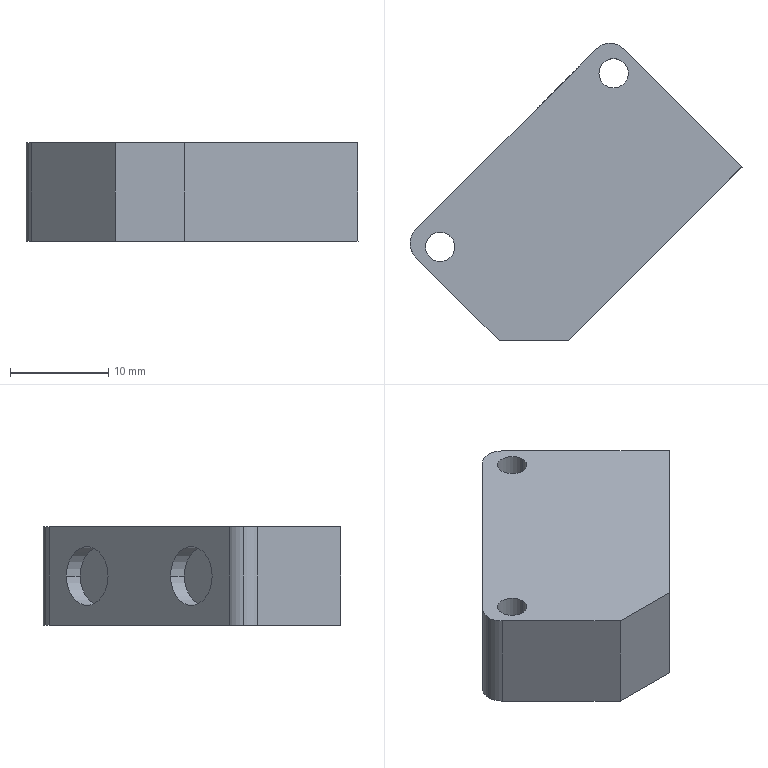Part | SolidWorks | features BaseBody 1 | 1 solid | 20 faces | box 33.82 x 30.284 x 10 mm | volume 5303 mm3 | cylinder 11 | plane 9 | commonest cylinder face diameters 3 x4 6 x4 4 x3
STEP:
#1=CARTESIAN_POINT('',(390.202,1591.211,-336.822));
#2=VERTEX_POINT('',#1);
#3=CARTESIAN_POINT('',(387.202,1591.211,-336.822));
#4=VERTEX_POINT('',#3);
#5=CARTESIAN_POINT('',(388.702,1591.211,-336.822));
#6=DIRECTION('',(0.,0.,-1.));
#7=DIRECTION('',(-1.,0.,0.));
#8=AXIS2_PLACEMENT_3D('',#5,#6,#7);
#9=CIRCLE('',#8,1.5);
#10=EDGE_CURVE('',#2,#4,#9,.T.);
#11=ORIENTED_EDGE('',*,*,#10,.F.);
#12=CARTESIAN_POINT('',(390.202,1591.211,-346.822));
#13=VERTEX_POINT('',#12);
#14=CARTESIAN_POINT('',(390.202,1591.211,-336.822));
#15=DIRECTION('',(0.,0.,-1.));
#16=VECTOR('',#15,1000.);
#17=LINE('',#14,#16);
#18=EDGE_CURVE('',#2,#13,#17,.T.);
#19=ORIENTED_EDGE('',*,*,#18,.T.);
#20=CARTESIAN_POINT('',(387.202,1591.211,-346.822));
#21=VERTEX_POINT('',#20);
#22=CARTESIAN_POINT('',(388.702,1591.211,-346.822));
#23=DIRECTION('',(0.,0.,-1.));
#24=DIRECTION('',(-1.,0.,0.));
#25=AXIS2_PLACEMENT_3D('',#22,#23,#24);
#26=CIRCLE('',#25,1.5);
#27=EDGE_CURVE('',#13,#21,#26,.T.);
#28=ORIENTED_EDGE('',*,*,#27,.T.);
#29=CARTESIAN_POINT('',(387.202,1591.211,-336.822));
#30=DIRECTION('',(0.,0.,-1.));
#31=VECTOR('',#30,1000.);
#32=LINE('',#29,#31);
#33=EDGE_CURVE('',#4,#21,#32,.T.);
#34=ORIENTED_EDGE('',*,*,#33,.F.);
#35=EDGE_LOOP('',(#11,#19,#28,#34));
#36=FACE_OUTER_BOUND('',#35,.T.);
#37=CARTESIAN_POINT('',(388.702,1591.211,-336.822));
#38=DIRECTION('',(0.,0.,-1.));
#39=DIRECTION('',(-1.,0.,0.));
#40=AXIS2_PLACEMENT_3D('',#37,#38,#39);
#41=CYLINDRICAL_SURFACE('',#40,1.5);
#42=ADVANCED_FACE('',(#36),#41,.F.);
#43=CARTESIAN_POINT('',(407.879,1608.889,-336.822));
#44=VERTEX_POINT('',#43);
#45=CARTESIAN_POINT('',(404.879,1608.889,-336.822));
#46=VERTEX_POINT('',#45);
#47=CARTESIAN_POINT('',(406.379,1608.889,-336.822));
#48=DIRECTION('',(0.,0.,-1.));
#49=DIRECTION('',(-1.,0.,0.));
#50=AXIS2_PLACEMENT_3D('',#47,#48,#49);
#51=CIRCLE('',#50,1.5);
#52=EDGE_CURVE('',#44,#46,#51,.T.);
#53=ORIENTED_EDGE('',*,*,#52,.F.);
#54=CARTESIAN_POINT('',(407.879,1608.889,-346.822));
#55=VERTEX_POINT('',#54);
#56=CARTESIAN_POINT('',(407.879,1608.889,-336.822));
#57=DIRECTION('',(0.,0.,-1.));
#58=VECTOR('',#57,1000.);
#59=LINE('',#56,#58);
#60=EDGE_CURVE('',#44,#55,#59,.T.);
#61=ORIENTED_EDGE('',*,*,#60,.T.);
#62=CARTESIAN_POINT('',(404.879,1608.889,-346.822));
#63=VERTEX_POINT('',#62);
#64=CARTESIAN_POINT('',(406.379,1608.889,-346.822));
#65=DIRECTION('',(0.,0.,-1.));
#66=DIRECTION('',(-1.,0.,0.));
#67=AXIS2_PLACEMENT_3D('',#64,#65,#66);
#68=CIRCLE('',#67,1.5);
#69=EDGE_CURVE('',#55,#63,#68,.T.);
#70=ORIENTED_EDGE('',*,*,#69,.T.);
#71=CARTESIAN_POINT('',(404.879,1608.889,-336.822));
#72=DIRECTION('',(0.,0.,-1.));
#73=VECTOR('',#72,1000.);
#74=LINE('',#71,#73);
#75=EDGE_CURVE('',#46,#63,#74,.T.);
#76=ORIENTED_EDGE('',*,*,#75,.F.);
#77=EDGE_LOOP('',(#53,#61,#70,#76));
#78=FACE_OUTER_BOUND('',#77,.T.);
#79=CARTESIAN_POINT('',(406.379,1608.889,-336.822));
#80=DIRECTION('',(0.,0.,-1.));
#81=DIRECTION('',(-1.,0.,0.));
#82=AXIS2_PLACEMENT_3D('',#79,#80,#81);
#83=CYLINDRICAL_SURFACE('',#82,1.5);
#84=ADVANCED_FACE('',(#78),#83,.F.);
#85=CARTESIAN_POINT('',(386.227,1590.151,-336.822));
#86=VERTEX_POINT('',#85);
#87=CARTESIAN_POINT('',(385.641,1591.565,-336.822));
#88=VERTEX_POINT('',#87);
#89=CARTESIAN_POINT('',(387.641,1591.565,-336.822));
#90=DIRECTION('',(0.,0.,-1.));
#91=DIRECTION('',(-1.,0.,0.));
#92=AXIS2_PLACEMENT_3D('',#89,#90,#91);
#93=CIRCLE('',#92,2.);
#94=EDGE_CURVE('',#86,#88,#93,.T.);
#95=ORIENTED_EDGE('',*,*,#94,.T.);
#96=CARTESIAN_POINT('',(385.641,1591.565,-346.822));
#97=VERTEX_POINT('',#96);
#98=CARTESIAN_POINT('',(385.641,1591.565,-336.822));
#99=DIRECTION('',(0.,0.,-1.));
#100=VECTOR('',#99,1000.);
#101=LINE('',#98,#100);
#102=EDGE_CURVE('',#88,#97,#101,.T.);
#103=ORIENTED_EDGE('',*,*,#102,.T.);
#104=CARTESIAN_POINT('',(386.227,1590.151,-346.822));
#105=VERTEX_POINT('',#104);
#106=CARTESIAN_POINT('',(387.641,1591.565,-346.822));
#107=DIRECTION('',(0.,0.,1.));
#108=DIRECTION('',(-1.,0.,0.));
#109=AXIS2_PLACEMENT_3D('',#106,#107,#108);
#110=CIRCLE('',#109,2.);
#111=EDGE_CURVE('',#97,#105,#110,.T.);
#112=ORIENTED_EDGE('',*,*,#111,.T.);
#113=CARTESIAN_POINT('',(386.227,1590.151,-336.822));
#114=DIRECTION('',(0.,0.,1.));
#115=VECTOR('',#114,1000.);
#116=LINE('',#113,#115);
#117=EDGE_CURVE('',#105,#86,#116,.T.);
#118=ORIENTED_EDGE('',*,*,#117,.T.);
#119=EDGE_LOOP('',(#95,#103,#112,#118));
#120=FACE_OUTER_BOUND('',#119,.T.);
#121=CARTESIAN_POINT('',(387.641,1591.565,-336.822));
#122=DIRECTION('',(0.,0.,-1.));
#123=DIRECTION('',(-1.,0.,0.));
#124=AXIS2_PLACEMENT_3D('',#121,#122,#123);
#125=CYLINDRICAL_SURFACE('',#124,2.);
#126=ADVANCED_FACE('',(#120),#125,.T.);
#127=CARTESIAN_POINT('',(404.258,1608.182,-341.822));
#128=VERTEX_POINT('',#127);
#129=CARTESIAN_POINT('',(400.015,1603.939,-341.822));
#130=VERTEX_POINT('',#129);
#131=CARTESIAN_POINT('',(402.137,1606.061,-341.822));
#132=DIRECTION('',(-0.7071,0.7071,0.));
#133=DIRECTION('',(-0.7071,-0.7071,0.));
#134=AXIS2_PLACEMENT_3D('',#131,#132,#133);
#135=CIRCLE('',#134,3.);
#136=EDGE_CURVE('',#128,#130,#135,.T.);
#137=ORIENTED_EDGE('',*,*,#136,.F.);
#138=CARTESIAN_POINT('',(402.844,1609.596,-341.822));
#139=VERTEX_POINT('',#138);
#140=CARTESIAN_POINT('',(404.258,1608.182,-341.822));
#141=DIRECTION('',(-0.7071,0.7071,0.));
#142=VECTOR('',#141,1000.);
#143=LINE('',#140,#142);
#144=EDGE_CURVE('',#128,#139,#143,.T.);
#145=ORIENTED_EDGE('',*,*,#144,.T.);
#146=CARTESIAN_POINT('',(398.601,1605.353,-341.822));
#147=VERTEX_POINT('',#146);
#148=CARTESIAN_POINT('',(400.722,1607.475,-341.822));
#149=DIRECTION('',(-0.7071,0.7071,0.));
#150=DIRECTION('',(-0.7071,-0.7071,0.));
#151=AXIS2_PLACEMENT_3D('',#148,#149,#150);
#152=CIRCLE('',#151,3.);
#153=EDGE_CURVE('',#139,#147,#152,.T.);
#154=ORIENTED_EDGE('',*,*,#153,.T.);
#155=CARTESIAN_POINT('',(400.015,1603.939,-341.822));
#156=DIRECTION('',(-0.7071,0.7071,0.));
#157=VECTOR('',#156,1000.);
#158=LINE('',#155,#157);
#159=EDGE_CURVE('',#130,#147,#158,.T.);
#160=ORIENTED_EDGE('',*,*,#159,.F.);
#161=EDGE_LOOP('',(#137,#145,#154,#160));
#162=FACE_OUTER_BOUND('',#161,.T.);
#163=CARTESIAN_POINT('',(402.137,1606.061,-341.822));
#164=DIRECTION('',(-0.7071,0.7071,0.));
#165=DIRECTION('',(-0.7071,-0.7071,0.));
#166=AXIS2_PLACEMENT_3D('',#163,#164,#165);
#167=CYLINDRICAL_SURFACE('',#166,3.);
#168=ADVANCED_FACE('',(#162),#167,.F.);
#169=CARTESIAN_POINT('',(393.651,1597.575,-341.822));
#170=VERTEX_POINT('',#169);
#171=CARTESIAN_POINT('',(389.409,1593.333,-341.822));
#172=VERTEX_POINT('',#171);
#173=CARTESIAN_POINT('',(391.53,1595.454,-341.822));
#174=DIRECTION('',(-0.7071,0.7071,0.));
#175=DIRECTION('',(-0.7071,-0.7071,0.));
#176=AXIS2_PLACEMENT_3D('',#173,#174,#175);
#177=CIRCLE('',#176,3.);
#178=EDGE_CURVE('',#170,#172,#177,.T.);
#179=ORIENTED_EDGE('',*,*,#178,.F.);
#180=CARTESIAN_POINT('',(392.237,1598.989,-341.822));
#181=VERTEX_POINT('',#180);
#182=CARTESIAN_POINT('',(393.651,1597.575,-341.822));
#183=DIRECTION('',(-0.7071,0.7071,0.));
#184=VECTOR('',#183,1000.);
#185=LINE('',#182,#184);
#186=EDGE_CURVE('',#170,#181,#185,.T.);
#187=ORIENTED_EDGE('',*,*,#186,.T.);
#188=CARTESIAN_POINT('',(387.994,1594.747,-341.822));
#189=VERTEX_POINT('',#188);
#190=CARTESIAN_POINT('',(390.116,1596.868,-341.822));
#191=DIRECTION('',(-0.7071,0.7071,0.));
#192=DIRECTION('',(-0.7071,-0.7071,0.));
#193=AXIS2_PLACEMENT_3D('',#190,#191,#192);
#194=CIRCLE('',#193,3.);
#195=EDGE_CURVE('',#181,#189,#194,.T.);
#196=ORIENTED_EDGE('',*,*,#195,.T.);
#197=CARTESIAN_POINT('',(389.409,1593.333,-341.822));
#198=DIRECTION('',(-0.7071,0.7071,0.));
#199=VECTOR('',#198,1000.);
#200=LINE('',#197,#199);
#201=EDGE_CURVE('',#172,#189,#200,.T.);
#202=ORIENTED_EDGE('',*,*,#201,.F.);
#203=EDGE_LOOP('',(#179,#187,#196,#202));
#204=FACE_OUTER_BOUND('',#203,.T.);
#205=CARTESIAN_POINT('',(391.53,1595.454,-341.822));
#206=DIRECTION('',(-0.7071,0.7071,0.));
#207=DIRECTION('',(-0.7071,-0.7071,0.));
#208=AXIS2_PLACEMENT_3D('',#205,#206,#207);
#209=CYLINDRICAL_SURFACE('',#208,3.);
#210=ADVANCED_FACE('',(#204),#209,.F.);
#211=CARTESIAN_POINT('',(388.702,1591.211,-346.822));
#212=DIRECTION('',(0.,0.,-1.));
#213=DIRECTION('',(-1.,0.,0.));
#214=AXIS2_PLACEMENT_3D('',#211,#212,#213);
#215=CIRCLE('',#214,1.5);
#216=EDGE_CURVE('',#21,#13,#215,.T.);
#217=ORIENTED_EDGE('',*,*,#216,.F.);
#218=ORIENTED_EDGE('',*,*,#27,.F.);
#219=EDGE_LOOP('',(#217,#218));
#220=FACE_BOUND('',#219,.T.);
#221=CARTESIAN_POINT('',(406.379,1608.889,-346.822));
#222=DIRECTION('',(0.,0.,-1.));
#223=DIRECTION('',(-1.,0.,0.));
#224=AXIS2_PLACEMENT_3D('',#221,#222,#223);
#225=CIRCLE('',#224,1.5);
#226=EDGE_CURVE('',#63,#55,#225,.T.);
#227=ORIENTED_EDGE('',*,*,#226,.F.);
#228=ORIENTED_EDGE('',*,*,#69,.F.);
#229=EDGE_LOOP('',(#227,#228));
#230=FACE_BOUND('',#229,.T.);
#231=CARTESIAN_POINT('',(401.783,1581.665,-346.822));
#232=VERTEX_POINT('',#231);
#233=CARTESIAN_POINT('',(419.461,1599.343,-346.822));
#234=VERTEX_POINT('',#233);
#235=CARTESIAN_POINT('',(401.783,1581.665,-346.822));
#236=DIRECTION('',(0.7071,0.7071,0.));
#237=VECTOR('',#236,1000.);
#238=LINE('',#235,#237);
#239=EDGE_CURVE('',#232,#234,#238,.T.);
#240=ORIENTED_EDGE('',*,*,#239,.F.);
#241=CARTESIAN_POINT('',(394.712,1581.665,-346.822));
#242=VERTEX_POINT('',#241);
#243=CARTESIAN_POINT('',(406.026,1581.665,-346.822));
#244=DIRECTION('',(1.,0.,0.));
#245=VECTOR('',#244,1000.);
#246=LINE('',#243,#245);
#247=EDGE_CURVE('',#242,#232,#246,.T.);
#248=ORIENTED_EDGE('',*,*,#247,.F.);
#249=CARTESIAN_POINT('',(386.227,1590.151,-346.822));
#250=DIRECTION('',(0.7071,-0.7071,0.));
#251=VECTOR('',#250,1000.);
#252=LINE('',#249,#251);
#253=EDGE_CURVE('',#105,#242,#252,.T.);
#254=ORIENTED_EDGE('',*,*,#253,.F.);
#255=ORIENTED_EDGE('',*,*,#111,.F.);
#256=CARTESIAN_POINT('',(386.227,1592.979,-346.822));
#257=VERTEX_POINT('',#256);
#258=CARTESIAN_POINT('',(387.641,1591.565,-346.822));
#259=DIRECTION('',(0.,0.,1.));
#260=DIRECTION('',(-1.,0.,0.));
#261=AXIS2_PLACEMENT_3D('',#258,#259,#260);
#262=CIRCLE('',#261,2.);
#263=EDGE_CURVE('',#257,#97,#262,.T.);
#264=ORIENTED_EDGE('',*,*,#263,.F.);
#265=CARTESIAN_POINT('',(404.612,1611.364,-346.822));
#266=VERTEX_POINT('',#265);
#267=CARTESIAN_POINT('',(404.612,1611.364,-346.822));
#268=DIRECTION('',(-0.7071,-0.7071,0.));
#269=VECTOR('',#268,1000.);
#270=LINE('',#267,#269);
#271=EDGE_CURVE('',#266,#257,#270,.T.);
#272=ORIENTED_EDGE('',*,*,#271,.F.);
#273=CARTESIAN_POINT('',(407.44,1611.364,-346.822));
#274=VERTEX_POINT('',#273);
#275=CARTESIAN_POINT('',(406.026,1609.95,-346.822));
#276=DIRECTION('',(0.,0.,1.));
#277=DIRECTION('',(-1.,0.,0.));
#278=AXIS2_PLACEMENT_3D('',#275,#276,#277);
#279=CIRCLE('',#278,2.);
#280=EDGE_CURVE('',#274,#266,#279,.T.);
#281=ORIENTED_EDGE('',*,*,#280,.F.);
#282=CARTESIAN_POINT('',(419.461,1599.343,-346.822));
#283=DIRECTION('',(-0.7071,0.7071,0.));
#284=VECTOR('',#283,1000.);
#285=LINE('',#282,#284);
#286=EDGE_CURVE('',#234,#274,#285,.T.);
#287=ORIENTED_EDGE('',*,*,#286,.F.);
#288=EDGE_LOOP('',(#240,#248,#254,#255,#264,#272,#281,#287));
#289=FACE_OUTER_BOUND('',#288,.T.);
#290=CARTESIAN_POINT('',(406.026,1609.95,-346.822));
#291=DIRECTION('',(0.,0.,1.));
#292=DIRECTION('',(1.,0.,0.));
#293=AXIS2_PLACEMENT_3D('',#290,#291,#292);
#294=PLANE('',#293);
#295=ADVANCED_FACE('',(#220,#230,#289),#294,.F.);
#296=ORIENTED_EDGE('',*,*,#18,.F.);
#297=CARTESIAN_POINT('',(388.702,1591.211,-336.822));
#298=DIRECTION('',(0.,0.,-1.));
#299=DIRECTION('',(-1.,0.,0.));
#300=AXIS2_PLACEMENT_3D('',#297,#298,#299);
#301=CIRCLE('',#300,1.5);
#302=EDGE_CURVE('',#4,#2,#301,.T.);
#303=ORIENTED_EDGE('',*,*,#302,.F.);
#304=ORIENTED_EDGE('',*,*,#33,.T.);
#305=ORIENTED_EDGE('',*,*,#216,.T.);
#306=EDGE_LOOP('',(#296,#303,#304,#305));
#307=FACE_OUTER_BOUND('',#306,.T.);
#308=CARTESIAN_POINT('',(388.702,1591.211,-336.822));
#309=DIRECTION('',(0.,0.,-1.));
#310=DIRECTION('',(-1.,0.,0.));
#311=AXIS2_PLACEMENT_3D('',#308,#309,#310);
#312=CYLINDRICAL_SURFACE('',#311,1.5);
#313=ADVANCED_FACE('',(#307),#312,.F.);
#314=ORIENTED_EDGE('',*,*,#60,.F.);
#315=CARTESIAN_POINT('',(406.379,1608.889,-336.822));
#316=DIRECTION('',(0.,0.,-1.));
#317=DIRECTION('',(-1.,0.,0.));
#318=AXIS2_PLACEMENT_3D('',#315,#316,#317);
#319=CIRCLE('',#318,1.5);
#320=EDGE_CURVE('',#46,#44,#319,.T.);
#321=ORIENTED_EDGE('',*,*,#320,.F.);
#322=ORIENTED_EDGE('',*,*,#75,.T.);
#323=ORIENTED_EDGE('',*,*,#226,.T.);
#324=EDGE_LOOP('',(#314,#321,#322,#323));
#325=FACE_OUTER_BOUND('',#324,.T.);
#326=CARTESIAN_POINT('',(406.379,1608.889,-336.822));
#327=DIRECTION('',(0.,0.,-1.));
#328=DIRECTION('',(-1.,0.,0.));
#329=AXIS2_PLACEMENT_3D('',#326,#327,#328);
#330=CYLINDRICAL_SURFACE('',#329,1.5);
#331=ADVANCED_FACE('',(#325),#330,.F.);
#332=CARTESIAN_POINT('',(419.461,1599.343,-336.822));
#333=VERTEX_POINT('',#332);
#334=CARTESIAN_POINT('',(407.44,1611.364,-336.822));
#335=VERTEX_POINT('',#334);
#336=CARTESIAN_POINT('',(407.44,1611.364,-336.822));
#337=DIRECTION('',(-0.7071,0.7071,0.));
#338=VECTOR('',#337,1000.);
#339=LINE('',#336,#338);
#340=EDGE_CURVE('',#333,#335,#339,.T.);
#341=ORIENTED_EDGE('',*,*,#340,.F.);
#342=CARTESIAN_POINT('',(419.461,1599.343,-336.822));
#343=DIRECTION('',(0.,0.,1.));
#344=VECTOR('',#343,1000.);
#345=LINE('',#342,#344);
#346=EDGE_CURVE('',#234,#333,#345,.T.);
#347=ORIENTED_EDGE('',*,*,#346,.F.);
#348=ORIENTED_EDGE('',*,*,#286,.T.);
#349=CARTESIAN_POINT('',(407.44,1611.364,-336.822));
#350=DIRECTION('',(0.,0.,-1.));
#351=VECTOR('',#350,1000.);
#352=LINE('',#349,#351);
#353=EDGE_CURVE('',#335,#274,#352,.T.);
#354=ORIENTED_EDGE('',*,*,#353,.F.);
#355=EDGE_LOOP('',(#341,#347,#348,#354));
#356=FACE_OUTER_BOUND('',#355,.T.);
#357=CARTESIAN_POINT('',(407.44,1611.364,-336.822));
#358=DIRECTION('',(-0.7071,-0.7071,0.));
#359=DIRECTION('',(0.7071,-0.7071,0.));
#360=AXIS2_PLACEMENT_3D('',#357,#358,#359);
#361=PLANE('',#360);
#362=ADVANCED_FACE('',(#356),#361,.F.);
#363=CARTESIAN_POINT('',(401.783,1581.665,-336.822));
#364=VERTEX_POINT('',#363);
#365=CARTESIAN_POINT('',(419.461,1599.343,-336.822));
#366=DIRECTION('',(0.7071,0.7071,0.));
#367=VECTOR('',#366,1000.);
#368=LINE('',#365,#367);
#369=EDGE_CURVE('',#364,#333,#368,.T.);
#370=ORIENTED_EDGE('',*,*,#369,.F.);
#371=CARTESIAN_POINT('',(401.783,1581.665,-336.822));
#372=DIRECTION('',(0.,0.,1.));
#373=VECTOR('',#372,1000.);
#374=LINE('',#371,#373);
#375=EDGE_CURVE('',#232,#364,#374,.T.);
#376=ORIENTED_EDGE('',*,*,#375,.F.);
#377=ORIENTED_EDGE('',*,*,#239,.T.);
#378=ORIENTED_EDGE('',*,*,#346,.T.);
#379=EDGE_LOOP('',(#370,#376,#377,#378));
#380=FACE_OUTER_BOUND('',#379,.T.);
#381=CARTESIAN_POINT('',(419.461,1599.343,-336.822));
#382=DIRECTION('',(-0.7071,0.7071,0.));
#383=DIRECTION('',(-0.7071,-0.7071,0.));
#384=AXIS2_PLACEMENT_3D('',#381,#382,#383);
#385=PLANE('',#384);
#386=ADVANCED_FACE('',(#380),#385,.F.);
#387=CARTESIAN_POINT('',(394.712,1581.665,-336.822));
#388=VERTEX_POINT('',#387);
#389=CARTESIAN_POINT('',(401.783,1581.665,-336.822));
#390=DIRECTION('',(1.,0.,0.));
#391=VECTOR('',#390,1000.);
#392=LINE('',#389,#391);
#393=EDGE_CURVE('',#388,#364,#392,.T.);
#394=ORIENTED_EDGE('',*,*,#393,.F.);
#395=CARTESIAN_POINT('',(394.712,1581.665,-336.822));
#396=DIRECTION('',(0.,0.,1.));
#397=VECTOR('',#396,1000.);
#398=LINE('',#395,#397);
#399=EDGE_CURVE('',#242,#388,#398,.T.);
#400=ORIENTED_EDGE('',*,*,#399,.F.);
#401=ORIENTED_EDGE('',*,*,#247,.T.);
#402=ORIENTED_EDGE('',*,*,#375,.T.);
#403=EDGE_LOOP('',(#394,#400,#401,#402));
#404=FACE_OUTER_BOUND('',#403,.T.);
#405=CARTESIAN_POINT('',(401.783,1581.665,-336.822));
#406=DIRECTION('',(0.,1.,0.));
#407=DIRECTION('',(-1.,0.,0.));
#408=AXIS2_PLACEMENT_3D('',#405,#406,#407);
#409=PLANE('',#408);
#410=ADVANCED_FACE('',(#404),#409,.F.);
#411=CARTESIAN_POINT('',(394.712,1581.665,-336.822));
#412=DIRECTION('',(0.7071,-0.7071,0.));
#413=VECTOR('',#412,1000.);
#414=LINE('',#411,#413);
#415=EDGE_CURVE('',#86,#388,#414,.T.);
#416=ORIENTED_EDGE('',*,*,#415,.F.);
#417=ORIENTED_EDGE('',*,*,#117,.F.);
#418=ORIENTED_EDGE('',*,*,#253,.T.);
#419=ORIENTED_EDGE('',*,*,#399,.T.);
#420=EDGE_LOOP('',(#416,#417,#418,#419));
#421=FACE_OUTER_BOUND('',#420,.T.);
#422=CARTESIAN_POINT('',(394.712,1581.665,-336.822));
#423=DIRECTION('',(0.7071,0.7071,0.));
#424=DIRECTION('',(-0.7071,0.7071,0.));
#425=AXIS2_PLACEMENT_3D('',#422,#423,#424);
#426=PLANE('',#425);
#427=ADVANCED_FACE('',(#421),#426,.F.);
#428=ORIENTED_EDGE('',*,*,#102,.F.);
#429=CARTESIAN_POINT('',(386.227,1592.979,-336.822));
#430=VERTEX_POINT('',#429);
#431=CARTESIAN_POINT('',(387.641,1591.565,-336.822));
#432=DIRECTION('',(0.,0.,-1.));
#433=DIRECTION('',(-1.,0.,0.));
#434=AXIS2_PLACEMENT_3D('',#431,#432,#433);
#435=CIRCLE('',#434,2.);
#436=EDGE_CURVE('',#88,#430,#435,.T.);
#437=ORIENTED_EDGE('',*,*,#436,.T.);
#438=CARTESIAN_POINT('',(386.227,1592.979,-336.822));
#439=DIRECTION('',(0.,0.,-1.));
#440=VECTOR('',#439,1000.);
#441=LINE('',#438,#440);
#442=EDGE_CURVE('',#430,#257,#441,.T.);
#443=ORIENTED_EDGE('',*,*,#442,.T.);
#444=ORIENTED_EDGE('',*,*,#263,.T.);
#445=EDGE_LOOP('',(#428,#437,#443,#444));
#446=FACE_OUTER_BOUND('',#445,.T.);
#447=CARTESIAN_POINT('',(387.641,1591.565,-336.822));
#448=DIRECTION('',(0.,0.,-1.));
#449=DIRECTION('',(-1.,0.,0.));
#450=AXIS2_PLACEMENT_3D('',#447,#448,#449);
#451=CYLINDRICAL_SURFACE('',#450,2.);
#452=ADVANCED_FACE('',(#446),#451,.T.);
#453=CARTESIAN_POINT('',(400.722,1607.475,-341.822));
#454=DIRECTION('',(-0.7071,0.7071,0.));
#455=DIRECTION('',(-0.7071,-0.7071,0.));
#456=AXIS2_PLACEMENT_3D('',#453,#454,#455);
#457=CIRCLE('',#456,3.);
#458=EDGE_CURVE('',#147,#139,#457,.T.);
#459=ORIENTED_EDGE('',*,*,#458,.F.);
#460=ORIENTED_EDGE('',*,*,#153,.F.);
#461=EDGE_LOOP('',(#459,#460));
#462=FACE_BOUND('',#461,.T.);
#463=CARTESIAN_POINT('',(390.116,1596.868,-341.822));
#464=DIRECTION('',(-0.7071,0.7071,0.));
#465=DIRECTION('',(-0.7071,-0.7071,0.));
#466=AXIS2_PLACEMENT_3D('',#463,#464,#465);
#467=CIRCLE('',#466,3.);
#468=EDGE_CURVE('',#189,#181,#467,.T.);
#469=ORIENTED_EDGE('',*,*,#468,.F.);
#470=ORIENTED_EDGE('',*,*,#195,.F.);
#471=EDGE_LOOP('',(#469,#470));
#472=FACE_BOUND('',#471,.T.);
#473=CARTESIAN_POINT('',(404.612,1611.364,-336.822));
#474=VERTEX_POINT('',#473);
#475=CARTESIAN_POINT('',(386.227,1592.979,-336.822));
#476=DIRECTION('',(-0.7071,-0.7071,0.));
#477=VECTOR('',#476,1000.);
#478=LINE('',#475,#477);
#479=EDGE_CURVE('',#474,#430,#478,.T.);
#480=ORIENTED_EDGE('',*,*,#479,.F.);
#481=CARTESIAN_POINT('',(404.612,1611.364,-336.822));
#482=DIRECTION('',(0.,0.,1.));
#483=VECTOR('',#482,1000.);
#484=LINE('',#481,#483);
#485=EDGE_CURVE('',#266,#474,#484,.T.);
#486=ORIENTED_EDGE('',*,*,#485,.F.);
#487=ORIENTED_EDGE('',*,*,#271,.T.);
#488=ORIENTED_EDGE('',*,*,#442,.F.);
#489=EDGE_LOOP('',(#480,#486,#487,#488));
#490=FACE_OUTER_BOUND('',#489,.T.);
#491=CARTESIAN_POINT('',(386.227,1592.979,-336.822));
#492=DIRECTION('',(0.7071,-0.7071,0.));
#493=DIRECTION('',(0.7071,0.7071,0.));
#494=AXIS2_PLACEMENT_3D('',#491,#492,#493);
#495=PLANE('',#494);
#496=ADVANCED_FACE('',(#462,#472,#490),#495,.F.);
#497=ORIENTED_EDGE('',*,*,#353,.T.);
#498=ORIENTED_EDGE('',*,*,#280,.T.);
#499=ORIENTED_EDGE('',*,*,#485,.T.);
#500=CARTESIAN_POINT('',(406.026,1609.95,-336.822));
#501=DIRECTION('',(0.,0.,-1.));
#502=DIRECTION('',(-1.,0.,0.));
#503=AXIS2_PLACEMENT_3D('',#500,#501,#502);
#504=CIRCLE('',#503,2.);
#505=EDGE_CURVE('',#474,#335,#504,.T.);
#506=ORIENTED_EDGE('',*,*,#505,.T.);
#507=EDGE_LOOP('',(#497,#498,#499,#506));
#508=FACE_OUTER_BOUND('',#507,.T.);
#509=CARTESIAN_POINT('',(406.026,1609.95,-336.822));
#510=DIRECTION('',(0.,0.,-1.));
#511=DIRECTION('',(-1.,0.,0.));
#512=AXIS2_PLACEMENT_3D('',#509,#510,#511);
#513=CYLINDRICAL_SURFACE('',#512,2.);
#514=ADVANCED_FACE('',(#508),#513,.T.);
#515=ORIENTED_EDGE('',*,*,#302,.T.);
#516=ORIENTED_EDGE('',*,*,#10,.T.);
#517=EDGE_LOOP('',(#515,#516));
#518=FACE_BOUND('',#517,.T.);
#519=ORIENTED_EDGE('',*,*,#320,.T.);
#520=ORIENTED_EDGE('',*,*,#52,.T.);
#521=EDGE_LOOP('',(#519,#520));
#522=FACE_BOUND('',#521,.T.);
#523=ORIENTED_EDGE('',*,*,#340,.T.);
#524=ORIENTED_EDGE('',*,*,#505,.F.);
#525=ORIENTED_EDGE('',*,*,#479,.T.);
#526=ORIENTED_EDGE('',*,*,#436,.F.);
#527=ORIENTED_EDGE('',*,*,#94,.F.);
#528=ORIENTED_EDGE('',*,*,#415,.T.);
#529=ORIENTED_EDGE('',*,*,#393,.T.);
#530=ORIENTED_EDGE('',*,*,#369,.T.);
#531=EDGE_LOOP('',(#523,#524,#525,#526,#527,#528,#529,#530));
#532=FACE_OUTER_BOUND('',#531,.T.);
#533=CARTESIAN_POINT('',(406.026,1609.95,-336.822));
#534=DIRECTION('',(0.,0.,1.));
#535=DIRECTION('',(1.,0.,0.));
#536=AXIS2_PLACEMENT_3D('',#533,#534,#535);
#537=PLANE('',#536);
#538=ADVANCED_FACE('',(#518,#522,#532),#537,.T.);
#539=ORIENTED_EDGE('',*,*,#144,.F.);
#540=CARTESIAN_POINT('',(402.137,1606.061,-341.822));
#541=DIRECTION('',(-0.7071,0.7071,0.));
#542=DIRECTION('',(-0.7071,-0.7071,0.));
#543=AXIS2_PLACEMENT_3D('',#540,#541,#542);
#544=CIRCLE('',#543,3.);
#545=EDGE_CURVE('',#130,#128,#544,.T.);
#546=ORIENTED_EDGE('',*,*,#545,.F.);
#547=ORIENTED_EDGE('',*,*,#159,.T.);
#548=ORIENTED_EDGE('',*,*,#458,.T.);
#549=EDGE_LOOP('',(#539,#546,#547,#548));
#550=FACE_OUTER_BOUND('',#549,.T.);
#551=CARTESIAN_POINT('',(402.137,1606.061,-341.822));
#552=DIRECTION('',(-0.7071,0.7071,0.));
#553=DIRECTION('',(-0.7071,-0.7071,0.));
#554=AXIS2_PLACEMENT_3D('',#551,#552,#553);
#555=CYLINDRICAL_SURFACE('',#554,3.);
#556=ADVANCED_FACE('',(#550),#555,.F.);
#557=ORIENTED_EDGE('',*,*,#186,.F.);
#558=CARTESIAN_POINT('',(391.53,1595.454,-341.822));
#559=DIRECTION('',(-0.7071,0.7071,0.));
#560=DIRECTION('',(-0.7071,-0.7071,0.));
#561=AXIS2_PLACEMENT_3D('',#558,#559,#560);
#562=CIRCLE('',#561,3.);
#563=EDGE_CURVE('',#172,#170,#562,.T.);
#564=ORIENTED_EDGE('',*,*,#563,.F.);
#565=ORIENTED_EDGE('',*,*,#201,.T.);
#566=ORIENTED_EDGE('',*,*,#468,.T.);
#567=EDGE_LOOP('',(#557,#564,#565,#566));
#568=FACE_OUTER_BOUND('',#567,.T.);
#569=CARTESIAN_POINT('',(391.53,1595.454,-341.822));
#570=DIRECTION('',(-0.7071,0.7071,0.));
#571=DIRECTION('',(-0.7071,-0.7071,0.));
#572=AXIS2_PLACEMENT_3D('',#569,#570,#571);
#573=CYLINDRICAL_SURFACE('',#572,3.);
#574=ADVANCED_FACE('',(#568),#573,.F.);
#575=ORIENTED_EDGE('',*,*,#545,.T.);
#576=ORIENTED_EDGE('',*,*,#136,.T.);
#577=EDGE_LOOP('',(#575,#576));
#578=FACE_OUTER_BOUND('',#577,.T.);
#579=CARTESIAN_POINT('',(402.137,1606.061,-341.822));
#580=DIRECTION('',(-0.7071,0.7071,0.));
#581=DIRECTION('',(-0.7071,-0.7071,0.));
#582=AXIS2_PLACEMENT_3D('',#579,#580,#581);
#583=PLANE('',#582);
#584=ADVANCED_FACE('',(#578),#583,.T.);
#585=ORIENTED_EDGE('',*,*,#563,.T.);
#586=ORIENTED_EDGE('',*,*,#178,.T.);
#587=EDGE_LOOP('',(#585,#586));
#588=FACE_OUTER_BOUND('',#587,.T.);
#589=CARTESIAN_POINT('',(391.53,1595.454,-341.822));
#590=DIRECTION('',(-0.7071,0.7071,0.));
#591=DIRECTION('',(-0.7071,-0.7071,0.));
#592=AXIS2_PLACEMENT_3D('',#589,#590,#591);
#593=PLANE('',#592);
#594=ADVANCED_FACE('',(#588),#593,.T.);
#595=CLOSED_SHELL('',(#42,#84,#126,#168,#210,#295,#313,#331,#362,#386,#410,#427,#452,#496,#514,#538,#556,#574,#584,#594));
#596=MANIFOLD_SOLID_BREP('',#595);
#597=CARTESIAN_POINT('',(0.,0.,0.));
#598=DIRECTION('',(0.,0.,1.));
#599=DIRECTION('',(1.,0.,0.));
#600=AXIS2_PLACEMENT_3D('',#597,#598,#599);
#601=(LENGTH_UNIT()NAMED_UNIT(*)SI_UNIT(.MILLI.,.METRE.));
#602=UNCERTAINTY_MEASURE_WITH_UNIT(LENGTH_MEASURE(0.00001),#601,'','');
#603=(NAMED_UNIT(*)PLANE_ANGLE_UNIT()SI_UNIT($,.RADIAN.));
#604=(NAMED_UNIT(*)SI_UNIT($,.STERADIAN.)SOLID_ANGLE_UNIT());
#605=(GEOMETRIC_REPRESENTATION_CONTEXT(3)GLOBAL_UNCERTAINTY_ASSIGNED_CONTEXT((#602))GLOBAL_UNIT_ASSIGNED_CONTEXT((#601,#603,#604))REPRESENTATION_CONTEXT('',''));
#606=ADVANCED_BREP_SHAPE_REPRESENTATION('',(#596,#600),#605);